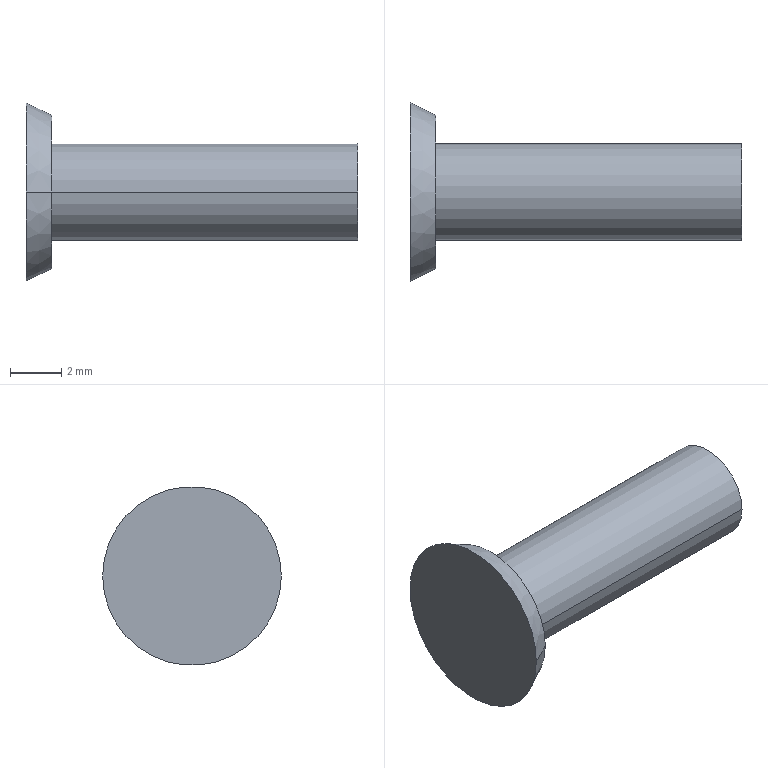Part | SolidWorks | features Revolution 1 | 1 solid | 7 faces | box 13 x 7 x 7 mm | volume 169.342 mm3 | plane 3 | cylinder 2 | cone 2 | commonest cylinder face diameters 3.8 x2
STEP:
#1=CARTESIAN_POINT('',(1.,1.9,0.));
#2=VERTEX_POINT('',#1);
#3=CARTESIAN_POINT('',(1.,-1.9,0.));
#4=VERTEX_POINT('',#3);
#5=CARTESIAN_POINT('',(1.,0.,0.));
#6=DIRECTION('',(1.,0.,0.));
#7=DIRECTION('',(0.,1.,0.));
#8=AXIS2_PLACEMENT_3D('',#5,#6,#7);
#9=CIRCLE('',#8,1.9);
#10=EDGE_CURVE('',#2,#4,#9,.T.);
#11=ORIENTED_EDGE('',*,*,#10,.T.);
#12=CARTESIAN_POINT('',(13.,-1.9,0.));
#13=VERTEX_POINT('',#12);
#14=CARTESIAN_POINT('',(13.,-1.9,0.));
#15=DIRECTION('',(1.,0.,0.));
#16=VECTOR('',#15,1000.);
#17=LINE('',#14,#16);
#18=EDGE_CURVE('',#4,#13,#17,.T.);
#19=ORIENTED_EDGE('',*,*,#18,.T.);
#20=CARTESIAN_POINT('',(13.,1.9,0.));
#21=VERTEX_POINT('',#20);
#22=CARTESIAN_POINT('',(13.,0.,0.));
#23=DIRECTION('',(1.,0.,0.));
#24=DIRECTION('',(0.,1.,0.));
#25=AXIS2_PLACEMENT_3D('',#22,#23,#24);
#26=CIRCLE('',#25,1.9);
#27=EDGE_CURVE('',#21,#13,#26,.T.);
#28=ORIENTED_EDGE('',*,*,#27,.F.);
#29=CARTESIAN_POINT('',(13.,1.9,0.));
#30=DIRECTION('',(1.,0.,0.));
#31=VECTOR('',#30,1000.);
#32=LINE('',#29,#31);
#33=EDGE_CURVE('',#2,#21,#32,.T.);
#34=ORIENTED_EDGE('',*,*,#33,.F.);
#35=EDGE_LOOP('',(#11,#19,#28,#34));
#36=FACE_OUTER_BOUND('',#35,.T.);
#37=CARTESIAN_POINT('',(13.,0.,0.));
#38=DIRECTION('',(1.,0.,0.));
#39=DIRECTION('',(0.,1.,0.));
#40=AXIS2_PLACEMENT_3D('',#37,#38,#39);
#41=CYLINDRICAL_SURFACE('',#40,1.9);
#42=ADVANCED_FACE('',(#36),#41,.T.);
#43=CARTESIAN_POINT('',(1.,3.,0.));
#44=VERTEX_POINT('',#43);
#45=CARTESIAN_POINT('',(1.,-3.,0.));
#46=VERTEX_POINT('',#45);
#47=CARTESIAN_POINT('',(1.,0.,0.));
#48=DIRECTION('',(1.,0.,0.));
#49=DIRECTION('',(0.,1.,0.));
#50=AXIS2_PLACEMENT_3D('',#47,#48,#49);
#51=CIRCLE('',#50,3.);
#52=EDGE_CURVE('',#44,#46,#51,.T.);
#53=ORIENTED_EDGE('',*,*,#52,.F.);
#54=CARTESIAN_POINT('',(0.,3.5,0.));
#55=VERTEX_POINT('',#54);
#56=CARTESIAN_POINT('',(1.,3.,0.));
#57=DIRECTION('',(-0.8944,0.4472,0.));
#58=VECTOR('',#57,1000.);
#59=LINE('',#56,#58);
#60=EDGE_CURVE('',#44,#55,#59,.T.);
#61=ORIENTED_EDGE('',*,*,#60,.T.);
#62=CARTESIAN_POINT('',(0.,-3.5,0.));
#63=VERTEX_POINT('',#62);
#64=CARTESIAN_POINT('',(0.,0.,0.));
#65=DIRECTION('',(1.,0.,0.));
#66=DIRECTION('',(0.,1.,0.));
#67=AXIS2_PLACEMENT_3D('',#64,#65,#66);
#68=CIRCLE('',#67,3.5);
#69=EDGE_CURVE('',#55,#63,#68,.T.);
#70=ORIENTED_EDGE('',*,*,#69,.T.);
#71=CARTESIAN_POINT('',(1.,-3.,0.));
#72=DIRECTION('',(-0.8944,-0.4472,0.));
#73=VECTOR('',#72,1000.);
#74=LINE('',#71,#73);
#75=EDGE_CURVE('',#46,#63,#74,.T.);
#76=ORIENTED_EDGE('',*,*,#75,.F.);
#77=EDGE_LOOP('',(#53,#61,#70,#76));
#78=FACE_OUTER_BOUND('',#77,.T.);
#79=CARTESIAN_POINT('',(1.,0.,0.));
#80=DIRECTION('',(-1.,0.,0.));
#81=DIRECTION('',(0.,-1.,0.));
#82=AXIS2_PLACEMENT_3D('',#79,#80,#81);
#83=CONICAL_SURFACE('',#82,3.,0.4636);
#84=ADVANCED_FACE('',(#78),#83,.T.);
#85=CARTESIAN_POINT('',(0.,0.,0.));
#86=DIRECTION('',(1.,0.,0.));
#87=DIRECTION('',(0.,1.,0.));
#88=AXIS2_PLACEMENT_3D('',#85,#86,#87);
#89=CIRCLE('',#88,3.5);
#90=EDGE_CURVE('',#63,#55,#89,.T.);
#91=ORIENTED_EDGE('',*,*,#90,.F.);
#92=ORIENTED_EDGE('',*,*,#69,.F.);
#93=EDGE_LOOP('',(#91,#92));
#94=FACE_OUTER_BOUND('',#93,.T.);
#95=CARTESIAN_POINT('',(0.,0.,0.));
#96=DIRECTION('',(-1.,0.,0.));
#97=DIRECTION('',(0.,-1.,0.));
#98=AXIS2_PLACEMENT_3D('',#95,#96,#97);
#99=PLANE('',#98);
#100=ADVANCED_FACE('',(#94),#99,.T.);
#101=ORIENTED_EDGE('',*,*,#60,.F.);
#102=CARTESIAN_POINT('',(1.,0.,0.));
#103=DIRECTION('',(1.,0.,0.));
#104=DIRECTION('',(0.,1.,0.));
#105=AXIS2_PLACEMENT_3D('',#102,#103,#104);
#106=CIRCLE('',#105,3.);
#107=EDGE_CURVE('',#46,#44,#106,.T.);
#108=ORIENTED_EDGE('',*,*,#107,.F.);
#109=ORIENTED_EDGE('',*,*,#75,.T.);
#110=ORIENTED_EDGE('',*,*,#90,.T.);
#111=EDGE_LOOP('',(#101,#108,#109,#110));
#112=FACE_OUTER_BOUND('',#111,.T.);
#113=CARTESIAN_POINT('',(1.,0.,0.));
#114=DIRECTION('',(-1.,0.,0.));
#115=DIRECTION('',(0.,-1.,0.));
#116=AXIS2_PLACEMENT_3D('',#113,#114,#115);
#117=CONICAL_SURFACE('',#116,3.,0.4636);
#118=ADVANCED_FACE('',(#112),#117,.T.);
#119=ORIENTED_EDGE('',*,*,#107,.T.);
#120=ORIENTED_EDGE('',*,*,#52,.T.);
#121=EDGE_LOOP('',(#119,#120));
#122=FACE_OUTER_BOUND('',#121,.T.);
#123=ORIENTED_EDGE('',*,*,#10,.F.);
#124=CARTESIAN_POINT('',(1.,0.,0.));
#125=DIRECTION('',(1.,0.,0.));
#126=DIRECTION('',(0.,1.,0.));
#127=AXIS2_PLACEMENT_3D('',#124,#125,#126);
#128=CIRCLE('',#127,1.9);
#129=EDGE_CURVE('',#4,#2,#128,.T.);
#130=ORIENTED_EDGE('',*,*,#129,.F.);
#131=EDGE_LOOP('',(#123,#130));
#132=FACE_BOUND('',#131,.T.);
#133=CARTESIAN_POINT('',(1.,3.,0.));
#134=DIRECTION('',(1.,0.,0.));
#135=DIRECTION('',(0.,1.,0.));
#136=AXIS2_PLACEMENT_3D('',#133,#134,#135);
#137=PLANE('',#136);
#138=ADVANCED_FACE('',(#122,#132),#137,.T.);
#139=ORIENTED_EDGE('',*,*,#18,.F.);
#140=ORIENTED_EDGE('',*,*,#129,.T.);
#141=ORIENTED_EDGE('',*,*,#33,.T.);
#142=CARTESIAN_POINT('',(13.,0.,0.));
#143=DIRECTION('',(1.,0.,0.));
#144=DIRECTION('',(0.,1.,0.));
#145=AXIS2_PLACEMENT_3D('',#142,#143,#144);
#146=CIRCLE('',#145,1.9);
#147=EDGE_CURVE('',#13,#21,#146,.T.);
#148=ORIENTED_EDGE('',*,*,#147,.F.);
#149=EDGE_LOOP('',(#139,#140,#141,#148));
#150=FACE_OUTER_BOUND('',#149,.T.);
#151=CARTESIAN_POINT('',(13.,0.,0.));
#152=DIRECTION('',(1.,0.,0.));
#153=DIRECTION('',(0.,1.,0.));
#154=AXIS2_PLACEMENT_3D('',#151,#152,#153);
#155=CYLINDRICAL_SURFACE('',#154,1.9);
#156=ADVANCED_FACE('',(#150),#155,.T.);
#157=ORIENTED_EDGE('',*,*,#27,.T.);
#158=ORIENTED_EDGE('',*,*,#147,.T.);
#159=EDGE_LOOP('',(#157,#158));
#160=FACE_OUTER_BOUND('',#159,.T.);
#161=CARTESIAN_POINT('',(13.,1.9,0.));
#162=DIRECTION('',(1.,0.,0.));
#163=DIRECTION('',(0.,1.,0.));
#164=AXIS2_PLACEMENT_3D('',#161,#162,#163);
#165=PLANE('',#164);
#166=ADVANCED_FACE('',(#160),#165,.T.);
#167=CLOSED_SHELL('',(#42,#84,#100,#118,#138,#156,#166));
#168=MANIFOLD_SOLID_BREP('',#167);
#169=CARTESIAN_POINT('',(0.,0.,0.));
#170=DIRECTION('',(0.,0.,1.));
#171=DIRECTION('',(1.,0.,0.));
#172=AXIS2_PLACEMENT_3D('',#169,#170,#171);
#173=(LENGTH_UNIT()NAMED_UNIT(*)SI_UNIT(.MILLI.,.METRE.));
#174=UNCERTAINTY_MEASURE_WITH_UNIT(LENGTH_MEASURE(0.00001),#173,'','');
#175=(NAMED_UNIT(*)PLANE_ANGLE_UNIT()SI_UNIT($,.RADIAN.));
#176=(NAMED_UNIT(*)SI_UNIT($,.STERADIAN.)SOLID_ANGLE_UNIT());
#177=(GEOMETRIC_REPRESENTATION_CONTEXT(3)GLOBAL_UNCERTAINTY_ASSIGNED_CONTEXT((#174))GLOBAL_UNIT_ASSIGNED_CONTEXT((#173,#175,#176))REPRESENTATION_CONTEXT('',''));
#178=ADVANCED_BREP_SHAPE_REPRESENTATION('',(#168,#172),#177);